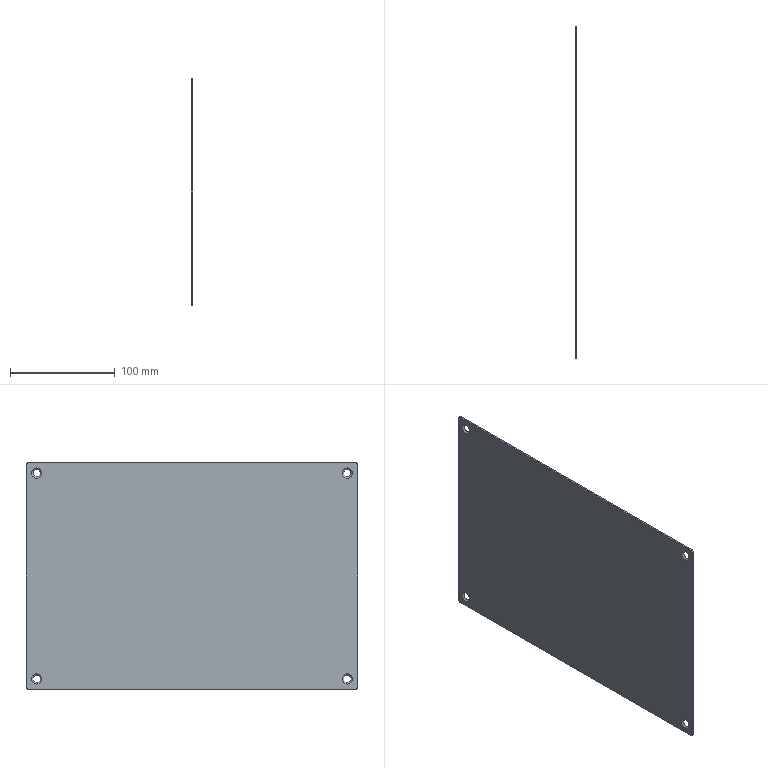Part | SolidWorks | features HoleWzd 2, Extrusion 1, Fillet 1 | 1 solid | 22 faces | box 1.5 x 316.6 x 216.5 mm | volume 102468 mm3 | cone 8 | cylinder 8 | plane 6 | commonest cylinder face diameters 6 x4 7.1 x4
STEP:
#1=CARTESIAN_POINT('',(2617.33,1359.3,89.095));
#2=VERTEX_POINT('',#1);
#3=CARTESIAN_POINT('',(2617.33,1359.3,96.195));
#4=VERTEX_POINT('',#3);
#5=CARTESIAN_POINT('',(2617.33,1359.3,92.645));
#6=DIRECTION('',(-1.,0.,0.));
#7=DIRECTION('',(0.,0.,1.));
#8=AXIS2_PLACEMENT_3D('',#5,#6,#7);
#9=CIRCLE('',#8,3.55);
#10=EDGE_CURVE('',#2,#4,#9,.T.);
#11=ORIENTED_EDGE('',*,*,#10,.F.);
#12=CARTESIAN_POINT('',(2615.93,1359.3,87.695));
#13=VERTEX_POINT('',#12);
#14=CARTESIAN_POINT('',(2615.93,1359.3,87.695));
#15=DIRECTION('',(-0.7071,0.,-0.7071));
#16=VECTOR('',#15,1000.);
#17=LINE('',#14,#16);
#18=EDGE_CURVE('',#2,#13,#17,.T.);
#19=ORIENTED_EDGE('',*,*,#18,.T.);
#20=CARTESIAN_POINT('',(2615.93,1359.3,97.595));
#21=VERTEX_POINT('',#20);
#22=CARTESIAN_POINT('',(2615.93,1359.3,92.645));
#23=DIRECTION('',(-1.,0.,0.));
#24=DIRECTION('',(0.,0.,1.));
#25=AXIS2_PLACEMENT_3D('',#22,#23,#24);
#26=CIRCLE('',#25,4.95);
#27=EDGE_CURVE('',#13,#21,#26,.T.);
#28=ORIENTED_EDGE('',*,*,#27,.T.);
#29=CARTESIAN_POINT('',(2615.93,1359.3,97.595));
#30=DIRECTION('',(-0.7071,0.,0.7071));
#31=VECTOR('',#30,1000.);
#32=LINE('',#29,#31);
#33=EDGE_CURVE('',#4,#21,#32,.T.);
#34=ORIENTED_EDGE('',*,*,#33,.F.);
#35=EDGE_LOOP('',(#11,#19,#28,#34));
#36=FACE_OUTER_BOUND('',#35,.T.);
#37=CARTESIAN_POINT('',(2615.93,1359.3,92.645));
#38=DIRECTION('',(-1.,0.,0.));
#39=DIRECTION('',(0.,0.,1.));
#40=AXIS2_PLACEMENT_3D('',#37,#38,#39);
#41=CONICAL_SURFACE('',#40,4.95,0.7854);
#42=ADVANCED_FACE('',(#36),#41,.F.);
#43=CARTESIAN_POINT('',(2617.43,1359.3,89.095));
#44=VERTEX_POINT('',#43);
#45=CARTESIAN_POINT('',(2617.43,1359.3,96.195));
#46=VERTEX_POINT('',#45);
#47=CARTESIAN_POINT('',(2617.43,1359.3,92.645));
#48=DIRECTION('',(-1.,0.,0.));
#49=DIRECTION('',(0.,0.,1.));
#50=AXIS2_PLACEMENT_3D('',#47,#48,#49);
#51=CIRCLE('',#50,3.55);
#52=EDGE_CURVE('',#44,#46,#51,.T.);
#53=ORIENTED_EDGE('',*,*,#52,.F.);
#54=CARTESIAN_POINT('',(2615.93,1359.3,89.095));
#55=DIRECTION('',(-1.,0.,0.));
#56=VECTOR('',#55,1000.);
#57=LINE('',#54,#56);
#58=EDGE_CURVE('',#44,#2,#57,.T.);
#59=ORIENTED_EDGE('',*,*,#58,.T.);
#60=ORIENTED_EDGE('',*,*,#10,.T.);
#61=CARTESIAN_POINT('',(2615.93,1359.3,96.195));
#62=DIRECTION('',(-1.,0.,0.));
#63=VECTOR('',#62,1000.);
#64=LINE('',#61,#63);
#65=EDGE_CURVE('',#46,#4,#64,.T.);
#66=ORIENTED_EDGE('',*,*,#65,.F.);
#67=EDGE_LOOP('',(#53,#59,#60,#66));
#68=FACE_OUTER_BOUND('',#67,.T.);
#69=CARTESIAN_POINT('',(2615.93,1359.3,92.645));
#70=DIRECTION('',(-1.,0.,0.));
#71=DIRECTION('',(0.,0.,1.));
#72=AXIS2_PLACEMENT_3D('',#69,#70,#71);
#73=CYLINDRICAL_SURFACE('',#72,3.55);
#74=ADVANCED_FACE('',(#68),#73,.F.);
#75=CARTESIAN_POINT('',(2617.33,1062.7,89.095));
#76=VERTEX_POINT('',#75);
#77=CARTESIAN_POINT('',(2617.33,1062.7,96.195));
#78=VERTEX_POINT('',#77);
#79=CARTESIAN_POINT('',(2617.33,1062.7,92.645));
#80=DIRECTION('',(-1.,0.,0.));
#81=DIRECTION('',(0.,0.,1.));
#82=AXIS2_PLACEMENT_3D('',#79,#80,#81);
#83=CIRCLE('',#82,3.55);
#84=EDGE_CURVE('',#76,#78,#83,.T.);
#85=ORIENTED_EDGE('',*,*,#84,.F.);
#86=CARTESIAN_POINT('',(2615.93,1062.7,87.695));
#87=VERTEX_POINT('',#86);
#88=CARTESIAN_POINT('',(2615.93,1062.7,87.695));
#89=DIRECTION('',(-0.7071,0.,-0.7071));
#90=VECTOR('',#89,1000.);
#91=LINE('',#88,#90);
#92=EDGE_CURVE('',#76,#87,#91,.T.);
#93=ORIENTED_EDGE('',*,*,#92,.T.);
#94=CARTESIAN_POINT('',(2615.93,1062.7,97.595));
#95=VERTEX_POINT('',#94);
#96=CARTESIAN_POINT('',(2615.93,1062.7,92.645));
#97=DIRECTION('',(-1.,0.,0.));
#98=DIRECTION('',(0.,0.,1.));
#99=AXIS2_PLACEMENT_3D('',#96,#97,#98);
#100=CIRCLE('',#99,4.95);
#101=EDGE_CURVE('',#87,#95,#100,.T.);
#102=ORIENTED_EDGE('',*,*,#101,.T.);
#103=CARTESIAN_POINT('',(2615.93,1062.7,97.595));
#104=DIRECTION('',(-0.7071,0.,0.7071));
#105=VECTOR('',#104,1000.);
#106=LINE('',#103,#105);
#107=EDGE_CURVE('',#78,#95,#106,.T.);
#108=ORIENTED_EDGE('',*,*,#107,.F.);
#109=EDGE_LOOP('',(#85,#93,#102,#108));
#110=FACE_OUTER_BOUND('',#109,.T.);
#111=CARTESIAN_POINT('',(2615.93,1062.7,92.645));
#112=DIRECTION('',(-1.,0.,0.));
#113=DIRECTION('',(0.,0.,1.));
#114=AXIS2_PLACEMENT_3D('',#111,#112,#113);
#115=CONICAL_SURFACE('',#114,4.95,0.7854);
#116=ADVANCED_FACE('',(#110),#115,.F.);
#117=CARTESIAN_POINT('',(2617.43,1062.7,89.095));
#118=VERTEX_POINT('',#117);
#119=CARTESIAN_POINT('',(2617.43,1062.7,96.195));
#120=VERTEX_POINT('',#119);
#121=CARTESIAN_POINT('',(2617.43,1062.7,92.645));
#122=DIRECTION('',(-1.,0.,0.));
#123=DIRECTION('',(0.,0.,1.));
#124=AXIS2_PLACEMENT_3D('',#121,#122,#123);
#125=CIRCLE('',#124,3.55);
#126=EDGE_CURVE('',#118,#120,#125,.T.);
#127=ORIENTED_EDGE('',*,*,#126,.F.);
#128=CARTESIAN_POINT('',(2615.93,1062.7,89.095));
#129=DIRECTION('',(-1.,0.,0.));
#130=VECTOR('',#129,1000.);
#131=LINE('',#128,#130);
#132=EDGE_CURVE('',#118,#76,#131,.T.);
#133=ORIENTED_EDGE('',*,*,#132,.T.);
#134=ORIENTED_EDGE('',*,*,#84,.T.);
#135=CARTESIAN_POINT('',(2615.93,1062.7,96.195));
#136=DIRECTION('',(-1.,0.,0.));
#137=VECTOR('',#136,1000.);
#138=LINE('',#135,#137);
#139=EDGE_CURVE('',#120,#78,#138,.T.);
#140=ORIENTED_EDGE('',*,*,#139,.F.);
#141=EDGE_LOOP('',(#127,#133,#134,#140));
#142=FACE_OUTER_BOUND('',#141,.T.);
#143=CARTESIAN_POINT('',(2615.93,1062.7,92.645));
#144=DIRECTION('',(-1.,0.,0.));
#145=DIRECTION('',(0.,0.,1.));
#146=AXIS2_PLACEMENT_3D('',#143,#144,#145);
#147=CYLINDRICAL_SURFACE('',#146,3.55);
#148=ADVANCED_FACE('',(#142),#147,.F.);
#149=CARTESIAN_POINT('',(2617.43,1062.7,285.695));
#150=VERTEX_POINT('',#149);
#151=CARTESIAN_POINT('',(2617.43,1062.7,292.595));
#152=VERTEX_POINT('',#151);
#153=CARTESIAN_POINT('',(2617.43,1062.7,289.145));
#154=DIRECTION('',(-1.,0.,0.));
#155=DIRECTION('',(0.,0.,1.));
#156=AXIS2_PLACEMENT_3D('',#153,#154,#155);
#157=CIRCLE('',#156,3.45);
#158=EDGE_CURVE('',#150,#152,#157,.T.);
#159=ORIENTED_EDGE('',*,*,#158,.F.);
#160=CARTESIAN_POINT('',(2615.93,1062.7,284.195));
#161=VERTEX_POINT('',#160);
#162=CARTESIAN_POINT('',(2615.93,1062.7,284.195));
#163=DIRECTION('',(-0.7071,0.,-0.7071));
#164=VECTOR('',#163,1000.);
#165=LINE('',#162,#164);
#166=EDGE_CURVE('',#150,#161,#165,.T.);
#167=ORIENTED_EDGE('',*,*,#166,.T.);
#168=CARTESIAN_POINT('',(2615.93,1062.7,294.095));
#169=VERTEX_POINT('',#168);
#170=CARTESIAN_POINT('',(2615.93,1062.7,289.145));
#171=DIRECTION('',(-1.,0.,0.));
#172=DIRECTION('',(0.,0.,1.));
#173=AXIS2_PLACEMENT_3D('',#170,#171,#172);
#174=CIRCLE('',#173,4.95);
#175=EDGE_CURVE('',#161,#169,#174,.T.);
#176=ORIENTED_EDGE('',*,*,#175,.T.);
#177=CARTESIAN_POINT('',(2615.93,1062.7,294.095));
#178=DIRECTION('',(-0.7071,0.,0.7071));
#179=VECTOR('',#178,1000.);
#180=LINE('',#177,#179);
#181=EDGE_CURVE('',#152,#169,#180,.T.);
#182=ORIENTED_EDGE('',*,*,#181,.F.);
#183=EDGE_LOOP('',(#159,#167,#176,#182));
#184=FACE_OUTER_BOUND('',#183,.T.);
#185=CARTESIAN_POINT('',(2615.93,1062.7,289.145));
#186=DIRECTION('',(-1.,0.,0.));
#187=DIRECTION('',(0.,0.,1.));
#188=AXIS2_PLACEMENT_3D('',#185,#186,#187);
#189=CONICAL_SURFACE('',#188,4.95,0.7854);
#190=ADVANCED_FACE('',(#184),#189,.F.);
#191=CARTESIAN_POINT('',(2617.43,1359.3,285.695));
#192=VERTEX_POINT('',#191);
#193=CARTESIAN_POINT('',(2617.43,1359.3,292.595));
#194=VERTEX_POINT('',#193);
#195=CARTESIAN_POINT('',(2617.43,1359.3,289.145));
#196=DIRECTION('',(-1.,0.,0.));
#197=DIRECTION('',(0.,0.,1.));
#198=AXIS2_PLACEMENT_3D('',#195,#196,#197);
#199=CIRCLE('',#198,3.45);
#200=EDGE_CURVE('',#192,#194,#199,.T.);
#201=ORIENTED_EDGE('',*,*,#200,.F.);
#202=CARTESIAN_POINT('',(2615.93,1359.3,284.195));
#203=VERTEX_POINT('',#202);
#204=CARTESIAN_POINT('',(2615.93,1359.3,284.195));
#205=DIRECTION('',(-0.7071,0.,-0.7071));
#206=VECTOR('',#205,1000.);
#207=LINE('',#204,#206);
#208=EDGE_CURVE('',#192,#203,#207,.T.);
#209=ORIENTED_EDGE('',*,*,#208,.T.);
#210=CARTESIAN_POINT('',(2615.93,1359.3,294.095));
#211=VERTEX_POINT('',#210);
#212=CARTESIAN_POINT('',(2615.93,1359.3,289.145));
#213=DIRECTION('',(-1.,0.,0.));
#214=DIRECTION('',(0.,0.,1.));
#215=AXIS2_PLACEMENT_3D('',#212,#213,#214);
#216=CIRCLE('',#215,4.95);
#217=EDGE_CURVE('',#203,#211,#216,.T.);
#218=ORIENTED_EDGE('',*,*,#217,.T.);
#219=CARTESIAN_POINT('',(2615.93,1359.3,294.095));
#220=DIRECTION('',(-0.7071,0.,0.7071));
#221=VECTOR('',#220,1000.);
#222=LINE('',#219,#221);
#223=EDGE_CURVE('',#194,#211,#222,.T.);
#224=ORIENTED_EDGE('',*,*,#223,.F.);
#225=EDGE_LOOP('',(#201,#209,#218,#224));
#226=FACE_OUTER_BOUND('',#225,.T.);
#227=CARTESIAN_POINT('',(2615.93,1359.3,289.145));
#228=DIRECTION('',(-1.,0.,0.));
#229=DIRECTION('',(0.,0.,1.));
#230=AXIS2_PLACEMENT_3D('',#227,#228,#229);
#231=CONICAL_SURFACE('',#230,4.95,0.7854);
#232=ADVANCED_FACE('',(#226),#231,.F.);
#233=CARTESIAN_POINT('',(2617.43,1055.7,299.145));
#234=VERTEX_POINT('',#233);
#235=CARTESIAN_POINT('',(2617.43,1366.3,299.145));
#236=VERTEX_POINT('',#235);
#237=CARTESIAN_POINT('',(2617.43,1052.7,299.145));
#238=DIRECTION('',(0.,1.,0.));
#239=VECTOR('',#238,1000.);
#240=LINE('',#237,#239);
#241=EDGE_CURVE('',#234,#236,#240,.T.);
#242=ORIENTED_EDGE('',*,*,#241,.T.);
#243=CARTESIAN_POINT('',(2615.93,1366.3,299.145));
#244=VERTEX_POINT('',#243);
#245=CARTESIAN_POINT('',(2617.43,1366.3,299.145));
#246=DIRECTION('',(-1.,0.,0.));
#247=VECTOR('',#246,1000.);
#248=LINE('',#245,#247);
#249=EDGE_CURVE('',#236,#244,#248,.T.);
#250=ORIENTED_EDGE('',*,*,#249,.T.);
#251=CARTESIAN_POINT('',(2615.93,1055.7,299.145));
#252=VERTEX_POINT('',#251);
#253=CARTESIAN_POINT('',(2615.93,1052.7,299.145));
#254=DIRECTION('',(0.,1.,0.));
#255=VECTOR('',#254,1000.);
#256=LINE('',#253,#255);
#257=EDGE_CURVE('',#252,#244,#256,.T.);
#258=ORIENTED_EDGE('',*,*,#257,.F.);
#259=CARTESIAN_POINT('',(2617.43,1055.7,299.145));
#260=DIRECTION('',(1.,0.,0.));
#261=VECTOR('',#260,1000.);
#262=LINE('',#259,#261);
#263=EDGE_CURVE('',#252,#234,#262,.T.);
#264=ORIENTED_EDGE('',*,*,#263,.T.);
#265=EDGE_LOOP('',(#242,#250,#258,#264));
#266=FACE_OUTER_BOUND('',#265,.T.);
#267=CARTESIAN_POINT('',(2617.43,1052.7,299.145));
#268=DIRECTION('',(0.,0.,1.));
#269=DIRECTION('',(1.,0.,0.));
#270=AXIS2_PLACEMENT_3D('',#267,#268,#269);
#271=PLANE('',#270);
#272=ADVANCED_FACE('',(#266),#271,.T.);
#273=CARTESIAN_POINT('',(2615.93,1052.7,85.645));
#274=VERTEX_POINT('',#273);
#275=CARTESIAN_POINT('',(2615.93,1052.7,296.145));
#276=VERTEX_POINT('',#275);
#277=CARTESIAN_POINT('',(2615.93,1052.7,82.645));
#278=DIRECTION('',(0.,0.,1.));
#279=VECTOR('',#278,1000.);
#280=LINE('',#277,#279);
#281=EDGE_CURVE('',#274,#276,#280,.T.);
#282=ORIENTED_EDGE('',*,*,#281,.F.);
#283=CARTESIAN_POINT('',(2617.43,1052.7,85.645));
#284=VERTEX_POINT('',#283);
#285=CARTESIAN_POINT('',(2617.43,1052.7,85.645));
#286=DIRECTION('',(1.,0.,0.));
#287=VECTOR('',#286,1000.);
#288=LINE('',#285,#287);
#289=EDGE_CURVE('',#274,#284,#288,.T.);
#290=ORIENTED_EDGE('',*,*,#289,.T.);
#291=CARTESIAN_POINT('',(2617.43,1052.7,296.145));
#292=VERTEX_POINT('',#291);
#293=CARTESIAN_POINT('',(2617.43,1052.7,82.645));
#294=DIRECTION('',(0.,0.,1.));
#295=VECTOR('',#294,1000.);
#296=LINE('',#293,#295);
#297=EDGE_CURVE('',#284,#292,#296,.T.);
#298=ORIENTED_EDGE('',*,*,#297,.T.);
#299=CARTESIAN_POINT('',(2617.43,1052.7,296.145));
#300=DIRECTION('',(-1.,0.,0.));
#301=VECTOR('',#300,1000.);
#302=LINE('',#299,#301);
#303=EDGE_CURVE('',#292,#276,#302,.T.);
#304=ORIENTED_EDGE('',*,*,#303,.T.);
#305=EDGE_LOOP('',(#282,#290,#298,#304));
#306=FACE_OUTER_BOUND('',#305,.T.);
#307=CARTESIAN_POINT('',(2617.43,1052.7,82.645));
#308=DIRECTION('',(0.,-1.,0.));
#309=DIRECTION('',(0.,0.,-1.));
#310=AXIS2_PLACEMENT_3D('',#307,#308,#309);
#311=PLANE('',#310);
#312=ADVANCED_FACE('',(#306),#311,.T.);
#313=CARTESIAN_POINT('',(2615.93,1366.3,82.645));
#314=VERTEX_POINT('',#313);
#315=CARTESIAN_POINT('',(2615.93,1055.7,82.645));
#316=VERTEX_POINT('',#315);
#317=CARTESIAN_POINT('',(2615.93,1369.3,82.645));
#318=DIRECTION('',(0.,-1.,0.));
#319=VECTOR('',#318,1000.);
#320=LINE('',#317,#319);
#321=EDGE_CURVE('',#314,#316,#320,.T.);
#322=ORIENTED_EDGE('',*,*,#321,.F.);
#323=CARTESIAN_POINT('',(2617.43,1366.3,82.645));
#324=VERTEX_POINT('',#323);
#325=CARTESIAN_POINT('',(2617.43,1366.3,82.645));
#326=DIRECTION('',(1.,0.,0.));
#327=VECTOR('',#326,1000.);
#328=LINE('',#325,#327);
#329=EDGE_CURVE('',#314,#324,#328,.T.);
#330=ORIENTED_EDGE('',*,*,#329,.T.);
#331=CARTESIAN_POINT('',(2617.43,1055.7,82.645));
#332=VERTEX_POINT('',#331);
#333=CARTESIAN_POINT('',(2617.43,1369.3,82.645));
#334=DIRECTION('',(0.,-1.,0.));
#335=VECTOR('',#334,1000.);
#336=LINE('',#333,#335);
#337=EDGE_CURVE('',#324,#332,#336,.T.);
#338=ORIENTED_EDGE('',*,*,#337,.T.);
#339=CARTESIAN_POINT('',(2617.43,1055.7,82.645));
#340=DIRECTION('',(-1.,0.,0.));
#341=VECTOR('',#340,1000.);
#342=LINE('',#339,#341);
#343=EDGE_CURVE('',#332,#316,#342,.T.);
#344=ORIENTED_EDGE('',*,*,#343,.T.);
#345=EDGE_LOOP('',(#322,#330,#338,#344));
#346=FACE_OUTER_BOUND('',#345,.T.);
#347=CARTESIAN_POINT('',(2617.43,1369.3,82.645));
#348=DIRECTION('',(0.,0.,-1.));
#349=DIRECTION('',(-1.,0.,0.));
#350=AXIS2_PLACEMENT_3D('',#347,#348,#349);
#351=PLANE('',#350);
#352=ADVANCED_FACE('',(#346),#351,.T.);
#353=CARTESIAN_POINT('',(2617.43,1369.3,296.145));
#354=VERTEX_POINT('',#353);
#355=CARTESIAN_POINT('',(2617.43,1369.3,85.645));
#356=VERTEX_POINT('',#355);
#357=CARTESIAN_POINT('',(2617.43,1369.3,299.145));
#358=DIRECTION('',(0.,0.,-1.));
#359=VECTOR('',#358,1000.);
#360=LINE('',#357,#359);
#361=EDGE_CURVE('',#354,#356,#360,.T.);
#362=ORIENTED_EDGE('',*,*,#361,.T.);
#363=CARTESIAN_POINT('',(2615.93,1369.3,85.645));
#364=VERTEX_POINT('',#363);
#365=CARTESIAN_POINT('',(2617.43,1369.3,85.645));
#366=DIRECTION('',(-1.,0.,0.));
#367=VECTOR('',#366,1000.);
#368=LINE('',#365,#367);
#369=EDGE_CURVE('',#356,#364,#368,.T.);
#370=ORIENTED_EDGE('',*,*,#369,.T.);
#371=CARTESIAN_POINT('',(2615.93,1369.3,296.145));
#372=VERTEX_POINT('',#371);
#373=CARTESIAN_POINT('',(2615.93,1369.3,299.145));
#374=DIRECTION('',(0.,0.,-1.));
#375=VECTOR('',#374,1000.);
#376=LINE('',#373,#375);
#377=EDGE_CURVE('',#372,#364,#376,.T.);
#378=ORIENTED_EDGE('',*,*,#377,.F.);
#379=CARTESIAN_POINT('',(2617.43,1369.3,296.145));
#380=DIRECTION('',(1.,0.,0.));
#381=VECTOR('',#380,1000.);
#382=LINE('',#379,#381);
#383=EDGE_CURVE('',#372,#354,#382,.T.);
#384=ORIENTED_EDGE('',*,*,#383,.T.);
#385=EDGE_LOOP('',(#362,#370,#378,#384));
#386=FACE_OUTER_BOUND('',#385,.T.);
#387=CARTESIAN_POINT('',(2617.43,1369.3,299.145));
#388=DIRECTION('',(0.,1.,0.));
#389=DIRECTION('',(0.,0.,1.));
#390=AXIS2_PLACEMENT_3D('',#387,#388,#389);
#391=PLANE('',#390);
#392=ADVANCED_FACE('',(#386),#391,.T.);
#393=CARTESIAN_POINT('',(2617.43,1359.3,92.645));
#394=DIRECTION('',(-1.,0.,0.));
#395=DIRECTION('',(0.,0.,1.));
#396=AXIS2_PLACEMENT_3D('',#393,#394,#395);
#397=CIRCLE('',#396,3.55);
#398=EDGE_CURVE('',#46,#44,#397,.T.);
#399=ORIENTED_EDGE('',*,*,#398,.T.);
#400=ORIENTED_EDGE('',*,*,#52,.T.);
#401=EDGE_LOOP('',(#399,#400));
#402=FACE_BOUND('',#401,.T.);
#403=CARTESIAN_POINT('',(2617.43,1062.7,92.645));
#404=DIRECTION('',(-1.,0.,0.));
#405=DIRECTION('',(0.,0.,1.));
#406=AXIS2_PLACEMENT_3D('',#403,#404,#405);
#407=CIRCLE('',#406,3.55);
#408=EDGE_CURVE('',#120,#118,#407,.T.);
#409=ORIENTED_EDGE('',*,*,#408,.T.);
#410=ORIENTED_EDGE('',*,*,#126,.T.);
#411=EDGE_LOOP('',(#409,#410));
#412=FACE_BOUND('',#411,.T.);
#413=CARTESIAN_POINT('',(2617.43,1062.7,289.145));
#414=DIRECTION('',(-1.,0.,0.));
#415=DIRECTION('',(0.,0.,1.));
#416=AXIS2_PLACEMENT_3D('',#413,#414,#415);
#417=CIRCLE('',#416,3.45);
#418=EDGE_CURVE('',#152,#150,#417,.T.);
#419=ORIENTED_EDGE('',*,*,#418,.T.);
#420=ORIENTED_EDGE('',*,*,#158,.T.);
#421=EDGE_LOOP('',(#419,#420));
#422=FACE_BOUND('',#421,.T.);
#423=CARTESIAN_POINT('',(2617.43,1359.3,289.145));
#424=DIRECTION('',(-1.,0.,0.));
#425=DIRECTION('',(0.,0.,1.));
#426=AXIS2_PLACEMENT_3D('',#423,#424,#425);
#427=CIRCLE('',#426,3.45);
#428=EDGE_CURVE('',#194,#192,#427,.T.);
#429=ORIENTED_EDGE('',*,*,#428,.T.);
#430=ORIENTED_EDGE('',*,*,#200,.T.);
#431=EDGE_LOOP('',(#429,#430));
#432=FACE_BOUND('',#431,.T.);
#433=ORIENTED_EDGE('',*,*,#337,.F.);
#434=CARTESIAN_POINT('',(2617.43,1366.3,85.645));
#435=DIRECTION('',(1.,0.,0.));
#436=DIRECTION('',(0.,0.,1.));
#437=AXIS2_PLACEMENT_3D('',#434,#435,#436);
#438=CIRCLE('',#437,3.);
#439=EDGE_CURVE('',#324,#356,#438,.T.);
#440=ORIENTED_EDGE('',*,*,#439,.T.);
#441=ORIENTED_EDGE('',*,*,#361,.F.);
#442=CARTESIAN_POINT('',(2617.43,1366.3,296.145));
#443=DIRECTION('',(1.,0.,0.));
#444=DIRECTION('',(0.,0.,1.));
#445=AXIS2_PLACEMENT_3D('',#442,#443,#444);
#446=CIRCLE('',#445,3.);
#447=EDGE_CURVE('',#354,#236,#446,.T.);
#448=ORIENTED_EDGE('',*,*,#447,.T.);
#449=ORIENTED_EDGE('',*,*,#241,.F.);
#450=CARTESIAN_POINT('',(2617.43,1055.7,296.145));
#451=DIRECTION('',(1.,0.,0.));
#452=DIRECTION('',(0.,0.,1.));
#453=AXIS2_PLACEMENT_3D('',#450,#451,#452);
#454=CIRCLE('',#453,3.);
#455=EDGE_CURVE('',#234,#292,#454,.T.);
#456=ORIENTED_EDGE('',*,*,#455,.T.);
#457=ORIENTED_EDGE('',*,*,#297,.F.);
#458=CARTESIAN_POINT('',(2617.43,1055.7,85.645));
#459=DIRECTION('',(1.,0.,0.));
#460=DIRECTION('',(0.,0.,1.));
#461=AXIS2_PLACEMENT_3D('',#458,#459,#460);
#462=CIRCLE('',#461,3.);
#463=EDGE_CURVE('',#284,#332,#462,.T.);
#464=ORIENTED_EDGE('',*,*,#463,.T.);
#465=EDGE_LOOP('',(#433,#440,#441,#448,#449,#456,#457,#464));
#466=FACE_OUTER_BOUND('',#465,.T.);
#467=CARTESIAN_POINT('',(2617.43,0.,0.));
#468=DIRECTION('',(-1.,0.,0.));
#469=DIRECTION('',(0.,0.,1.));
#470=AXIS2_PLACEMENT_3D('',#467,#468,#469);
#471=PLANE('',#470);
#472=ADVANCED_FACE('',(#402,#412,#422,#432,#466),#471,.F.);
#473=CARTESIAN_POINT('',(2615.93,1359.3,92.645));
#474=DIRECTION('',(-1.,0.,0.));
#475=DIRECTION('',(0.,0.,1.));
#476=AXIS2_PLACEMENT_3D('',#473,#474,#475);
#477=CIRCLE('',#476,4.95);
#478=EDGE_CURVE('',#21,#13,#477,.T.);
#479=ORIENTED_EDGE('',*,*,#478,.F.);
#480=ORIENTED_EDGE('',*,*,#27,.F.);
#481=EDGE_LOOP('',(#479,#480));
#482=FACE_BOUND('',#481,.T.);
#483=CARTESIAN_POINT('',(2615.93,1062.7,92.645));
#484=DIRECTION('',(-1.,0.,0.));
#485=DIRECTION('',(0.,0.,1.));
#486=AXIS2_PLACEMENT_3D('',#483,#484,#485);
#487=CIRCLE('',#486,4.95);
#488=EDGE_CURVE('',#95,#87,#487,.T.);
#489=ORIENTED_EDGE('',*,*,#488,.F.);
#490=ORIENTED_EDGE('',*,*,#101,.F.);
#491=EDGE_LOOP('',(#489,#490));
#492=FACE_BOUND('',#491,.T.);
#493=CARTESIAN_POINT('',(2615.93,1062.7,289.145));
#494=DIRECTION('',(-1.,0.,0.));
#495=DIRECTION('',(0.,0.,1.));
#496=AXIS2_PLACEMENT_3D('',#493,#494,#495);
#497=CIRCLE('',#496,4.95);
#498=EDGE_CURVE('',#169,#161,#497,.T.);
#499=ORIENTED_EDGE('',*,*,#498,.F.);
#500=ORIENTED_EDGE('',*,*,#175,.F.);
#501=EDGE_LOOP('',(#499,#500));
#502=FACE_BOUND('',#501,.T.);
#503=CARTESIAN_POINT('',(2615.93,1359.3,289.145));
#504=DIRECTION('',(-1.,0.,0.));
#505=DIRECTION('',(0.,0.,1.));
#506=AXIS2_PLACEMENT_3D('',#503,#504,#505);
#507=CIRCLE('',#506,4.95);
#508=EDGE_CURVE('',#211,#203,#507,.T.);
#509=ORIENTED_EDGE('',*,*,#508,.F.);
#510=ORIENTED_EDGE('',*,*,#217,.F.);
#511=EDGE_LOOP('',(#509,#510));
#512=FACE_BOUND('',#511,.T.);
#513=ORIENTED_EDGE('',*,*,#377,.T.);
#514=CARTESIAN_POINT('',(2615.93,1366.3,85.645));
#515=DIRECTION('',(-1.,0.,0.));
#516=DIRECTION('',(0.,0.,1.));
#517=AXIS2_PLACEMENT_3D('',#514,#515,#516);
#518=CIRCLE('',#517,3.);
#519=EDGE_CURVE('',#364,#314,#518,.T.);
#520=ORIENTED_EDGE('',*,*,#519,.T.);
#521=ORIENTED_EDGE('',*,*,#321,.T.);
#522=CARTESIAN_POINT('',(2615.93,1055.7,85.645));
#523=DIRECTION('',(-1.,0.,0.));
#524=DIRECTION('',(0.,0.,1.));
#525=AXIS2_PLACEMENT_3D('',#522,#523,#524);
#526=CIRCLE('',#525,3.);
#527=EDGE_CURVE('',#316,#274,#526,.T.);
#528=ORIENTED_EDGE('',*,*,#527,.T.);
#529=ORIENTED_EDGE('',*,*,#281,.T.);
#530=CARTESIAN_POINT('',(2615.93,1055.7,296.145));
#531=DIRECTION('',(-1.,0.,0.));
#532=DIRECTION('',(0.,0.,1.));
#533=AXIS2_PLACEMENT_3D('',#530,#531,#532);
#534=CIRCLE('',#533,3.);
#535=EDGE_CURVE('',#276,#252,#534,.T.);
#536=ORIENTED_EDGE('',*,*,#535,.T.);
#537=ORIENTED_EDGE('',*,*,#257,.T.);
#538=CARTESIAN_POINT('',(2615.93,1366.3,296.145));
#539=DIRECTION('',(-1.,0.,0.));
#540=DIRECTION('',(0.,0.,1.));
#541=AXIS2_PLACEMENT_3D('',#538,#539,#540);
#542=CIRCLE('',#541,3.);
#543=EDGE_CURVE('',#244,#372,#542,.T.);
#544=ORIENTED_EDGE('',*,*,#543,.T.);
#545=EDGE_LOOP('',(#513,#520,#521,#528,#529,#536,#537,#544));
#546=FACE_OUTER_BOUND('',#545,.T.);
#547=CARTESIAN_POINT('',(2615.93,0.,0.));
#548=DIRECTION('',(-1.,0.,0.));
#549=DIRECTION('',(0.,0.,1.));
#550=AXIS2_PLACEMENT_3D('',#547,#548,#549);
#551=PLANE('',#550);
#552=ADVANCED_FACE('',(#482,#492,#502,#512,#546),#551,.T.);
#553=ORIENTED_EDGE('',*,*,#208,.F.);
#554=ORIENTED_EDGE('',*,*,#428,.F.);
#555=ORIENTED_EDGE('',*,*,#223,.T.);
#556=ORIENTED_EDGE('',*,*,#508,.T.);
#557=EDGE_LOOP('',(#553,#554,#555,#556));
#558=FACE_OUTER_BOUND('',#557,.T.);
#559=CARTESIAN_POINT('',(2615.93,1359.3,289.145));
#560=DIRECTION('',(-1.,0.,0.));
#561=DIRECTION('',(0.,0.,1.));
#562=AXIS2_PLACEMENT_3D('',#559,#560,#561);
#563=CONICAL_SURFACE('',#562,4.95,0.7854);
#564=ADVANCED_FACE('',(#558),#563,.F.);
#565=ORIENTED_EDGE('',*,*,#166,.F.);
#566=ORIENTED_EDGE('',*,*,#418,.F.);
#567=ORIENTED_EDGE('',*,*,#181,.T.);
#568=ORIENTED_EDGE('',*,*,#498,.T.);
#569=EDGE_LOOP('',(#565,#566,#567,#568));
#570=FACE_OUTER_BOUND('',#569,.T.);
#571=CARTESIAN_POINT('',(2615.93,1062.7,289.145));
#572=DIRECTION('',(-1.,0.,0.));
#573=DIRECTION('',(0.,0.,1.));
#574=AXIS2_PLACEMENT_3D('',#571,#572,#573);
#575=CONICAL_SURFACE('',#574,4.95,0.7854);
#576=ADVANCED_FACE('',(#570),#575,.F.);
#577=ORIENTED_EDGE('',*,*,#132,.F.);
#578=ORIENTED_EDGE('',*,*,#408,.F.);
#579=ORIENTED_EDGE('',*,*,#139,.T.);
#580=CARTESIAN_POINT('',(2617.33,1062.7,92.645));
#581=DIRECTION('',(-1.,0.,0.));
#582=DIRECTION('',(0.,0.,1.));
#583=AXIS2_PLACEMENT_3D('',#580,#581,#582);
#584=CIRCLE('',#583,3.55);
#585=EDGE_CURVE('',#78,#76,#584,.T.);
#586=ORIENTED_EDGE('',*,*,#585,.T.);
#587=EDGE_LOOP('',(#577,#578,#579,#586));
#588=FACE_OUTER_BOUND('',#587,.T.);
#589=CARTESIAN_POINT('',(2615.93,1062.7,92.645));
#590=DIRECTION('',(-1.,0.,0.));
#591=DIRECTION('',(0.,0.,1.));
#592=AXIS2_PLACEMENT_3D('',#589,#590,#591);
#593=CYLINDRICAL_SURFACE('',#592,3.55);
#594=ADVANCED_FACE('',(#588),#593,.F.);
#595=ORIENTED_EDGE('',*,*,#92,.F.);
#596=ORIENTED_EDGE('',*,*,#585,.F.);
#597=ORIENTED_EDGE('',*,*,#107,.T.);
#598=ORIENTED_EDGE('',*,*,#488,.T.);
#599=EDGE_LOOP('',(#595,#596,#597,#598));
#600=FACE_OUTER_BOUND('',#599,.T.);
#601=CARTESIAN_POINT('',(2615.93,1062.7,92.645));
#602=DIRECTION('',(-1.,0.,0.));
#603=DIRECTION('',(0.,0.,1.));
#604=AXIS2_PLACEMENT_3D('',#601,#602,#603);
#605=CONICAL_SURFACE('',#604,4.95,0.7854);
#606=ADVANCED_FACE('',(#600),#605,.F.);
#607=ORIENTED_EDGE('',*,*,#58,.F.);
#608=ORIENTED_EDGE('',*,*,#398,.F.);
#609=ORIENTED_EDGE('',*,*,#65,.T.);
#610=CARTESIAN_POINT('',(2617.33,1359.3,92.645));
#611=DIRECTION('',(-1.,0.,0.));
#612=DIRECTION('',(0.,0.,1.));
#613=AXIS2_PLACEMENT_3D('',#610,#611,#612);
#614=CIRCLE('',#613,3.55);
#615=EDGE_CURVE('',#4,#2,#614,.T.);
#616=ORIENTED_EDGE('',*,*,#615,.T.);
#617=EDGE_LOOP('',(#607,#608,#609,#616));
#618=FACE_OUTER_BOUND('',#617,.T.);
#619=CARTESIAN_POINT('',(2615.93,1359.3,92.645));
#620=DIRECTION('',(-1.,0.,0.));
#621=DIRECTION('',(0.,0.,1.));
#622=AXIS2_PLACEMENT_3D('',#619,#620,#621);
#623=CYLINDRICAL_SURFACE('',#622,3.55);
#624=ADVANCED_FACE('',(#618),#623,.F.);
#625=ORIENTED_EDGE('',*,*,#18,.F.);
#626=ORIENTED_EDGE('',*,*,#615,.F.);
#627=ORIENTED_EDGE('',*,*,#33,.T.);
#628=ORIENTED_EDGE('',*,*,#478,.T.);
#629=EDGE_LOOP('',(#625,#626,#627,#628));
#630=FACE_OUTER_BOUND('',#629,.T.);
#631=CARTESIAN_POINT('',(2615.93,1359.3,92.645));
#632=DIRECTION('',(-1.,0.,0.));
#633=DIRECTION('',(0.,0.,1.));
#634=AXIS2_PLACEMENT_3D('',#631,#632,#633);
#635=CONICAL_SURFACE('',#634,4.95,0.7854);
#636=ADVANCED_FACE('',(#630),#635,.F.);
#637=ORIENTED_EDGE('',*,*,#439,.F.);
#638=ORIENTED_EDGE('',*,*,#329,.F.);
#639=ORIENTED_EDGE('',*,*,#519,.F.);
#640=ORIENTED_EDGE('',*,*,#369,.F.);
#641=EDGE_LOOP('',(#637,#638,#639,#640));
#642=FACE_OUTER_BOUND('',#641,.T.);
#643=CARTESIAN_POINT('',(2617.43,1366.3,85.645));
#644=DIRECTION('',(-1.,0.,0.));
#645=DIRECTION('',(0.,0.,1.));
#646=AXIS2_PLACEMENT_3D('',#643,#644,#645);
#647=CYLINDRICAL_SURFACE('',#646,3.);
#648=ADVANCED_FACE('',(#642),#647,.T.);
#649=ORIENTED_EDGE('',*,*,#463,.F.);
#650=ORIENTED_EDGE('',*,*,#289,.F.);
#651=ORIENTED_EDGE('',*,*,#527,.F.);
#652=ORIENTED_EDGE('',*,*,#343,.F.);
#653=EDGE_LOOP('',(#649,#650,#651,#652));
#654=FACE_OUTER_BOUND('',#653,.T.);
#655=CARTESIAN_POINT('',(2617.43,1055.7,85.645));
#656=DIRECTION('',(-1.,0.,0.));
#657=DIRECTION('',(0.,0.,1.));
#658=AXIS2_PLACEMENT_3D('',#655,#656,#657);
#659=CYLINDRICAL_SURFACE('',#658,3.);
#660=ADVANCED_FACE('',(#654),#659,.T.);
#661=ORIENTED_EDGE('',*,*,#447,.F.);
#662=ORIENTED_EDGE('',*,*,#383,.F.);
#663=ORIENTED_EDGE('',*,*,#543,.F.);
#664=ORIENTED_EDGE('',*,*,#249,.F.);
#665=EDGE_LOOP('',(#661,#662,#663,#664));
#666=FACE_OUTER_BOUND('',#665,.T.);
#667=CARTESIAN_POINT('',(2617.43,1366.3,296.145));
#668=DIRECTION('',(-1.,0.,0.));
#669=DIRECTION('',(0.,0.,1.));
#670=AXIS2_PLACEMENT_3D('',#667,#668,#669);
#671=CYLINDRICAL_SURFACE('',#670,3.);
#672=ADVANCED_FACE('',(#666),#671,.T.);
#673=ORIENTED_EDGE('',*,*,#455,.F.);
#674=ORIENTED_EDGE('',*,*,#263,.F.);
#675=ORIENTED_EDGE('',*,*,#535,.F.);
#676=ORIENTED_EDGE('',*,*,#303,.F.);
#677=EDGE_LOOP('',(#673,#674,#675,#676));
#678=FACE_OUTER_BOUND('',#677,.T.);
#679=CARTESIAN_POINT('',(2617.43,1055.7,296.145));
#680=DIRECTION('',(-1.,0.,0.));
#681=DIRECTION('',(0.,0.,1.));
#682=AXIS2_PLACEMENT_3D('',#679,#680,#681);
#683=CYLINDRICAL_SURFACE('',#682,3.);
#684=ADVANCED_FACE('',(#678),#683,.T.);
#685=CLOSED_SHELL('',(#42,#74,#116,#148,#190,#232,#272,#312,#352,#392,#472,#552,#564,#576,#594,#606,#624,#636,#648,#660,#672,#684));
#686=MANIFOLD_SOLID_BREP('',#685);
#687=CARTESIAN_POINT('',(0.,0.,0.));
#688=DIRECTION('',(0.,0.,1.));
#689=DIRECTION('',(1.,0.,0.));
#690=AXIS2_PLACEMENT_3D('',#687,#688,#689);
#691=(LENGTH_UNIT()NAMED_UNIT(*)SI_UNIT(.MILLI.,.METRE.));
#692=UNCERTAINTY_MEASURE_WITH_UNIT(LENGTH_MEASURE(0.00001),#691,'','');
#693=(NAMED_UNIT(*)PLANE_ANGLE_UNIT()SI_UNIT($,.RADIAN.));
#694=(NAMED_UNIT(*)SI_UNIT($,.STERADIAN.)SOLID_ANGLE_UNIT());
#695=(GEOMETRIC_REPRESENTATION_CONTEXT(3)GLOBAL_UNCERTAINTY_ASSIGNED_CONTEXT((#692))GLOBAL_UNIT_ASSIGNED_CONTEXT((#691,#693,#694))REPRESENTATION_CONTEXT('',''));
#696=ADVANCED_BREP_SHAPE_REPRESENTATION('',(#686,#690),#695);